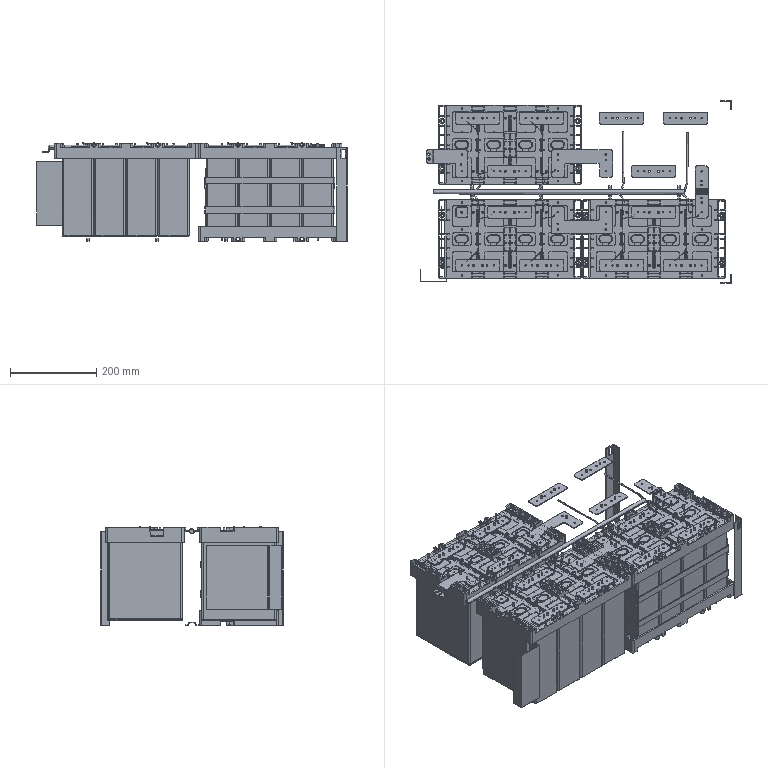Part | NX | features BREP 1 | 77 solids | 7761 faces | volume 31949023 mm3 | plane 4711 | cylinder 2536 | cone 304 | spline 120 | torus 86 | sphere 4 | commonest cylinder face diameters 6 x546 4 x506 10 x250 3 x196 2 x156 8 x128